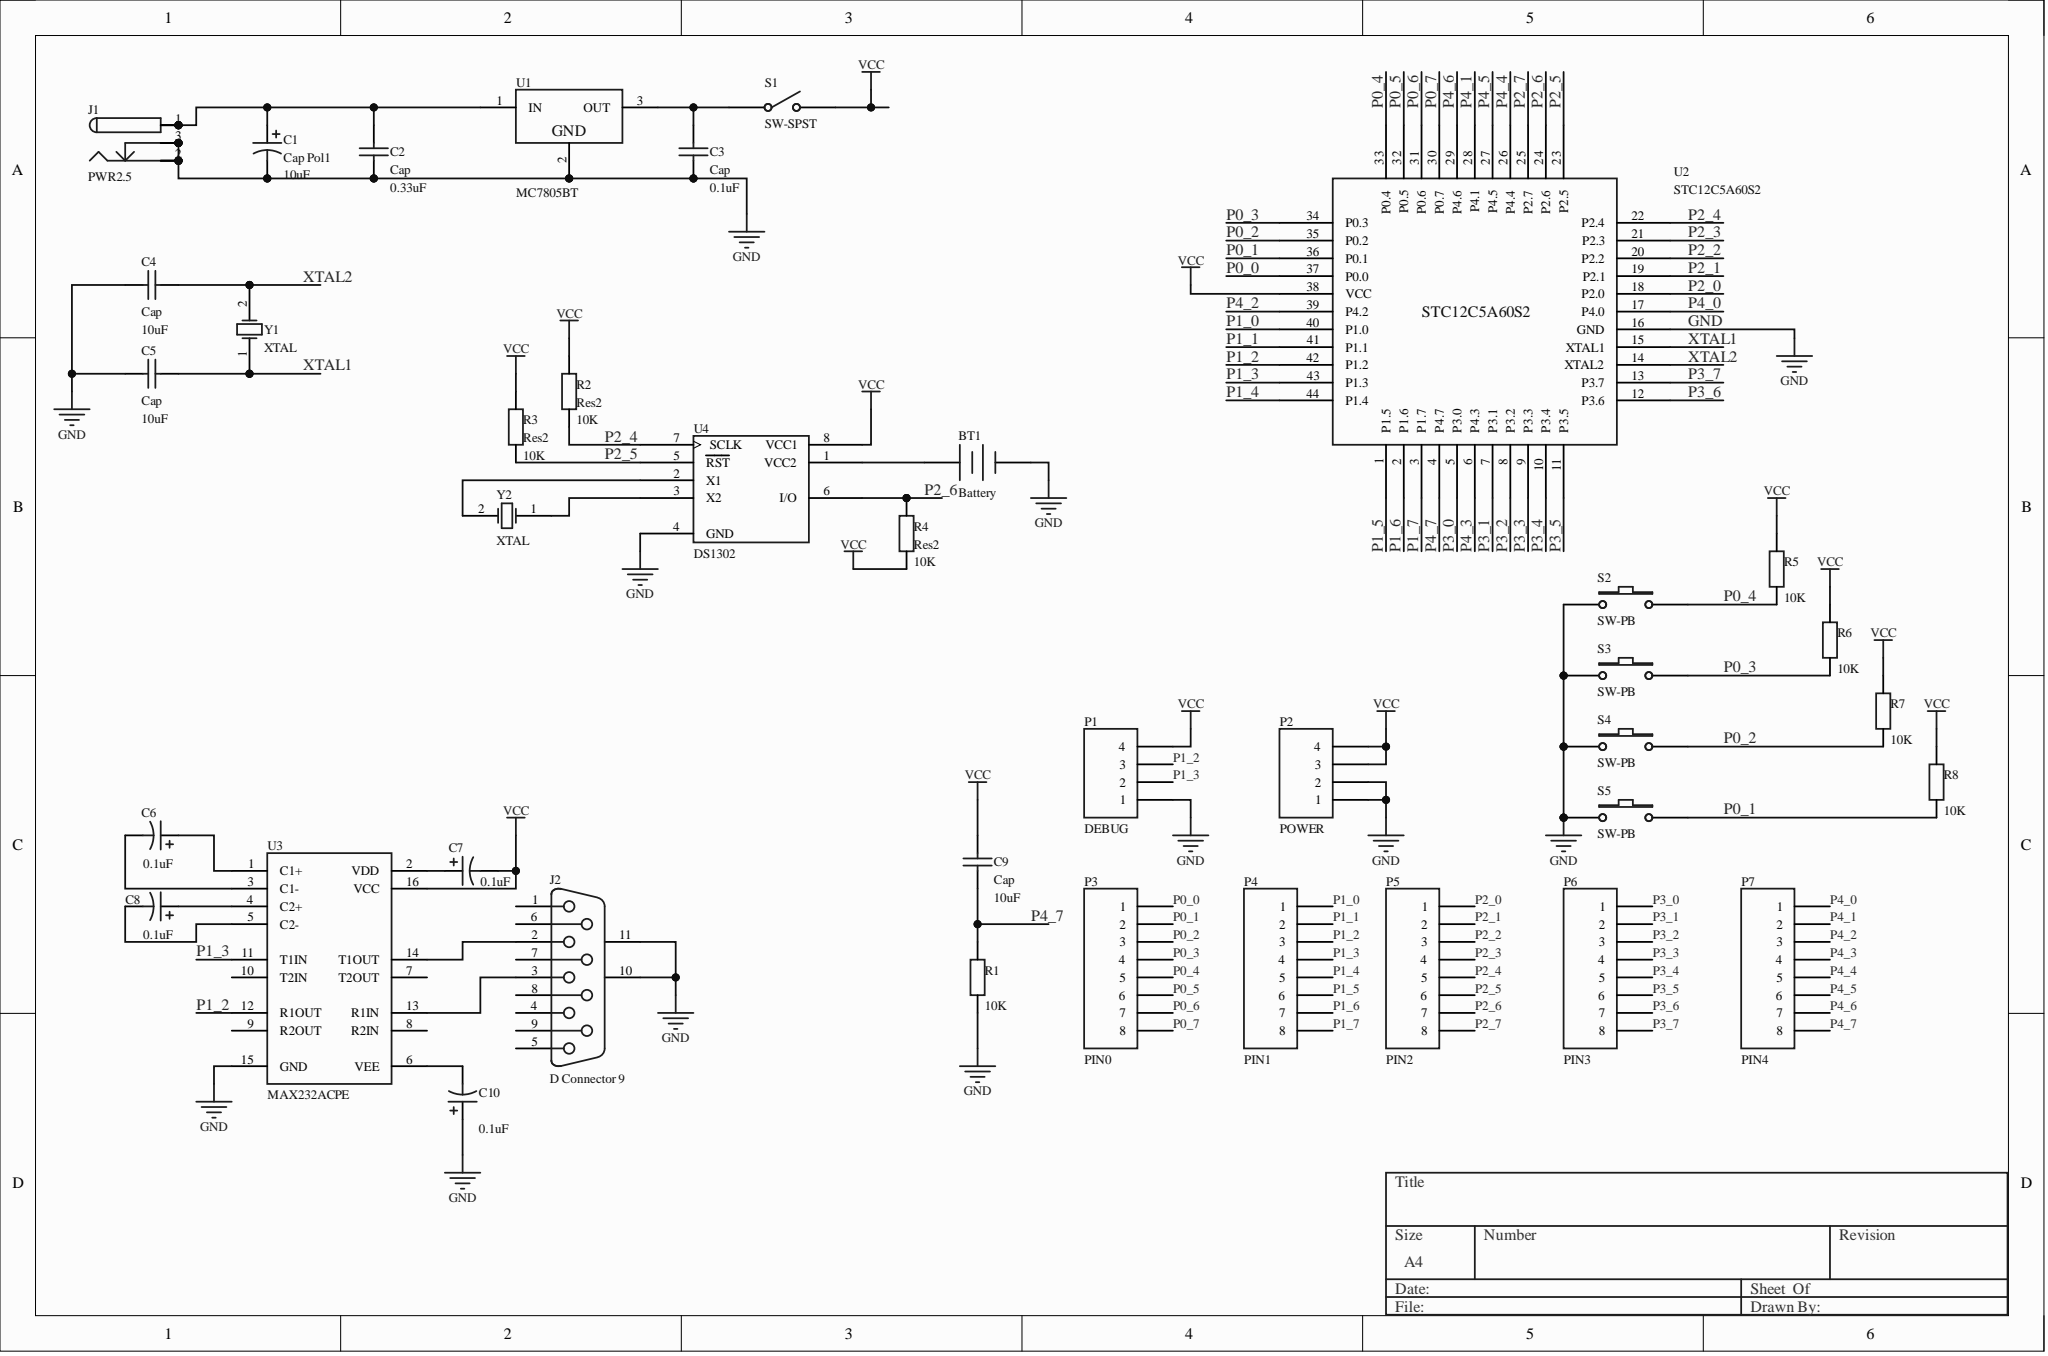Circuit board | Altium Designer | 39 parts | 57 nets
Bill of materials:
Comment,Description,Designator,Footprint,LibRef,Quantity
"Battery","Multicell Battery","BT1","BAT-2","Battery","1"
"Cap Pol1","Polarized Capacitor (Radial)","C1, C6, C7, C8, C10","RB2.54-5.08","Cap Pol1","5"
"Cap","Capacitor","C2","RAD-0.3","Cap","1"
"Cap","Capacitor","C3, C4, C5, C9","C0805","Cap","4"
"PWR2.5","Low Voltage Power Supply Connector","J1","KLD-0202","PWR2.5","1"
"D Connector 9","Receptacle Assembly, 9 Position, Right Angle","J2","DSUB1.385-2H9","D Connector 9","1"
"DEBUG","Header, 4-Pin","P1","HDR1X4","DEBUG","1"
"POWER","Header, 4-Pin","P2","HDR1X4","POWER","1"
"PIN0","Header, 8-Pin","P3","HDR1X8","PIN0","1"
"PIN1","Header, 8-Pin","P4","HDR1X8","PIN1","1"
"PIN2","Header, 8-Pin","P5","HDR1X8","PIN2","1"
"PIN3","Header, 8-Pin","P6","HDR1X8","PIN3","1"
"PIN4","Header, 8-Pin","P7","HDR1X8","PIN4","1"
"Res2","Resistor","R1, R2, R3, R4, R5, R6, R7, R8","6-0805_L","Res2","8"
"SW-SPST","Single-Pole, Single-Throw Switch","S1","SPST-2","SW-SPST","1"
"SW-PB","Switch","S2, S3, S4, S5","SPST-2","SW-PB","4"
"MC7805BT","3-Terminal Positive Fixed Voltage Regulator","U1","221A-04","MC7805BT","1"
"STC12C5A60S2","","U2","TQFP-44","STC12C5A60S2","1"
"MAX232ACPE","+5V Powered, Multi-Channel RS-232 Driver/Receiver","U3","PE16A","MAX232ACPE","1"
"DS1302","","U4","DIP-8","DS1302","1"
"XTAL","Crystal Oscillator","Y1, Y2","R38","XTAL","2"
Netlist (Protel format):
[
BT1
BAT-2
Battery



]
[
C1
RB2.54-5.08
Cap Pol1



]
[
C2
RAD-0.3
Cap



]
[
C3
C0805
Cap



]
[
C4
C0805
Cap



]
[
C5
C0805
Cap



]
[
C6
RB2.54-5.08
Cap Pol1



]
[
C7
RB2.54-5.08
Cap Pol1



]
[
C8
RB2.54-5.08
Cap Pol1



]
[
C9
C0805
Cap



]
[
C10
RB2.54-5.08
Cap Pol1



]
[
J1
KLD-0202
PWR2.5



]
[
J2
DSUB1.385-2H9
D Connector 9



]
[
P1
HDR1X4
DEBUG



]
[
P2
HDR1X4
POWER



]
[
P3
HDR1X8
PIN0



]
[
P4
HDR1X8
PIN1



]
[
P5
HDR1X8
PIN2



]
[
P6
HDR1X8
PIN3



]
[
P7
HDR1X8
PIN4



]
[
R1
6-0805_L
Res2



]
[
R2
6-0805_L
Res2



]
[
R3
6-0805_L
Res2



]
[
R4
6-0805_L
Res2



]
[
R5
6-0805_L
Res2



]
[
R6
6-0805_L
Res2



]
[
R7
6-0805_L
Res2



]
[
R8
6-0805_L
Res2



]
[
S1
SPST-2
SW-SPST



]
[
S2
SPST-2
SW-PB



]
[
S3
SPST-2
SW-PB



]
[
S4
SPST-2
SW-PB



]
[
S5
SPST-2
SW-PB



]
[
U1
221A-04
MC7805BT



]
[
U2
TQFP-44
STC12C5A60S2



]
[
U3
PE16A
MAX232ACPE



]
[
U4
DIP-8
DS1302



]
[
Y1
R38
XTAL



]
[
Y2
R38
XTAL



]
(
XTAL2
C4-1
U2-14
Y1-2
)
(
XTAL1
C5-1
U2-15
Y1-1
)
(
VCC
C7-2
C9-2
P1-4
P2-3
P2-4
R2-2
R3-2
R4-1
R5-2
R6-2
R7-2
R8-2
S1-2
U2-38
U3-16
U4-8
)
(
P4_7
C9-1
P7-8
R1-2
U2-4
)
(
P4_6
P7-7
U2-29
)
(
P4_5
P7-6
U2-27
)
(
P4_4
P7-5
U2-26
)
(
P4_3
P7-4
U2-6
)
(
P4_2
P7-3
U2-39
)
(
P4_1
P7-2
U2-28
)
(
P4_0
P7-1
U2-17
)
(
P3_7
P6-8
U2-13
)
(
P3_6
P6-7
U2-12
)
(
P3_5
P6-6
U2-11
)
(
P3_4
P6-5
U2-10
)
(
P3_3
P6-4
U2-9
)
(
P3_2
P6-3
U2-8
)
(
P3_1
P6-2
U2-7
)
(
P3_0
P6-1
U2-5
)
(
P2_7
P5-8
U2-25
)
(
P2_6
P5-7
R4-2
U2-24
U4-6
)
(
P2_5
P5-6
R3-1
U2-23
U4-5
)
(
P2_4
P5-5
R2-1
U2-22
U4-7
)
(
P2_3
P5-4
U2-21
)
(
P2_2
P5-3
U2-20
)
(
P2_1
P5-2
U2-19
)
(
P2_0
P5-1
U2-18
)
(
P1_7
P4-8
U2-3
)
(
P1_6
P4-7
U2-2
)
(
P1_5
P4-6
U2-1
)
(
P1_4
P4-5
U2-44
)
(
P1_3
P1-2
P4-4
U2-43
U3-11
)
(
P1_2
P1-3
P4-3
U2-42
U3-12
)
(
P1_1
P4-2
U2-41
)
(
P1_0
P4-1
U2-40
)
(
P0_7
P3-8
U2-30
)
(
P0_6
P3-7
U2-31
)
(
P0_5
P3-6
U2-32
)
(
P0_4
P3-5
R5-1
S2-2
U2-33
)
(
P0_3
P3-4
R6-1
S3-2
U2-34
)
(
P0_2
P3-3
R7-1
S4-2
U2-35
)
(
P0_1
P3-2
R8-1
S5-2
U2-36
)
(
P0_0
P3-1
U2-37
)
(
NetU4_3
U4-3
Y2-1
)
(
NetU4_2
U4-2
Y2-2
)
(
NetJ2_3
J2-3
U3-13
)
(
NetJ2_2
J2-2
U3-14
)
(
NetC10_2
C10-2
U3-6
)
(
NetC8_2
C8-2
U3-5
)
(
NetC8_1
C8-1
U3-4
)
(
NetC7_1
C7-1
U3-2
)
(
NetC6_2
C6-2
U3-3
)
(
NetC6_1
C6-1
U3-1
)
(
NetC3_2
C3-2
S1-1
U1-3
)
(
NetC1_1
C1-1
C2-2
J1-1
J1-1A
J1-1B
U1-1
)
(
NetBT1_1
BT1-1
U4-1
)
(
GND
BT1-2
C1-2
C2-1
C3-1
C4-2
C5-2
C10-1
J1-2
J1-2A
J1-2B
J1-3
J1-3A
J1-3B
J2-10
J2-11
P1-1
P2-1
P2-2
R1-1
S2-1
S3-1
S4-1
S5-1
U1-2
U2-16
U3-15
U4-4
)